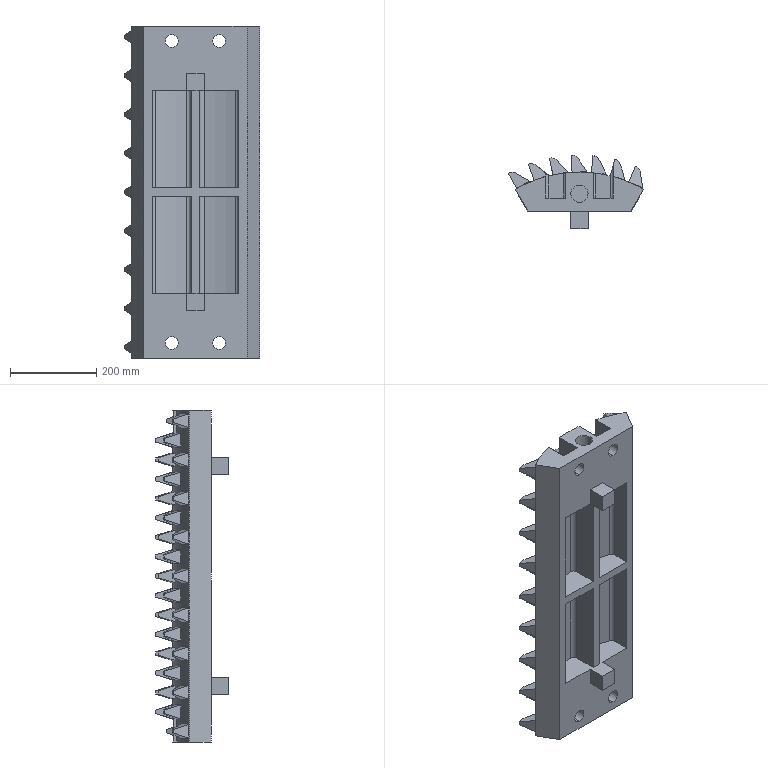Part | NX | features BREP 1 | 1 solid | 470 faces | box 313.534 x 169.472 x 770 mm | volume 12115990 mm3 | plane 381 | cylinder 89 | commonest cylinder face diameters 38 x56 10 x8 20 x8 30 x8 40 x4 550 x4